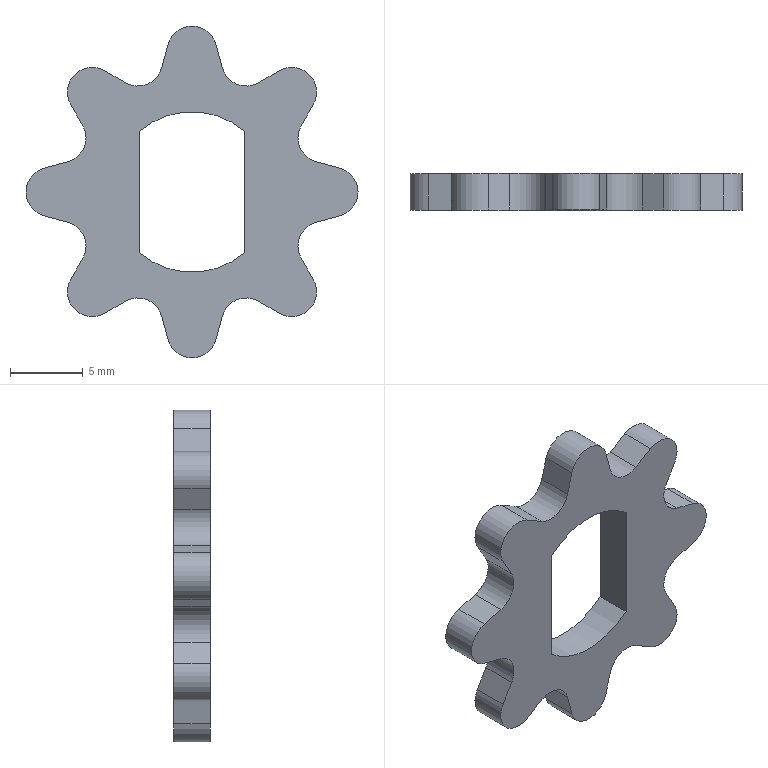Part | STEP file | _X2_751F4E45_X0_MS731-1_X2_8_25 | 1 solid | 38 faces | box 22.757 x 2.5 x 22.757 mm | volume 558.462 mm3 | plane 20 | cylinder 18 | commonest cylinder face diameters 3.4 x16 11 x2